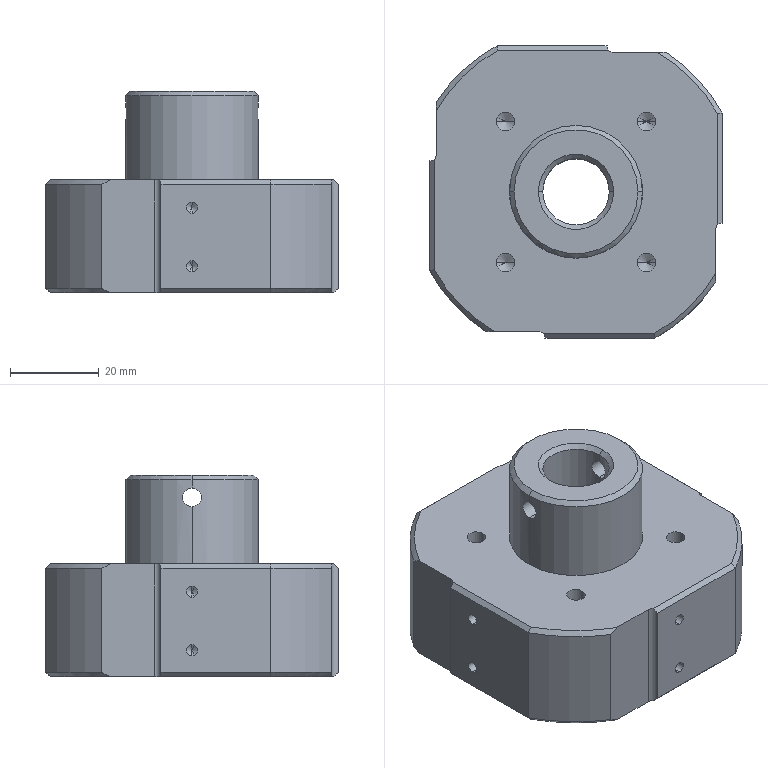Part | STEP file | 10000020580swp000-1 | 1 solid | 97 faces | box 66 x 66 x 45.5 mm | volume 104414 mm3 | cylinder 40 | cone 38 | plane 19 | commonest cylinder face diameters 2.5 x16 4.2 x12 3 x4 75 x4 15 x2 30 x2